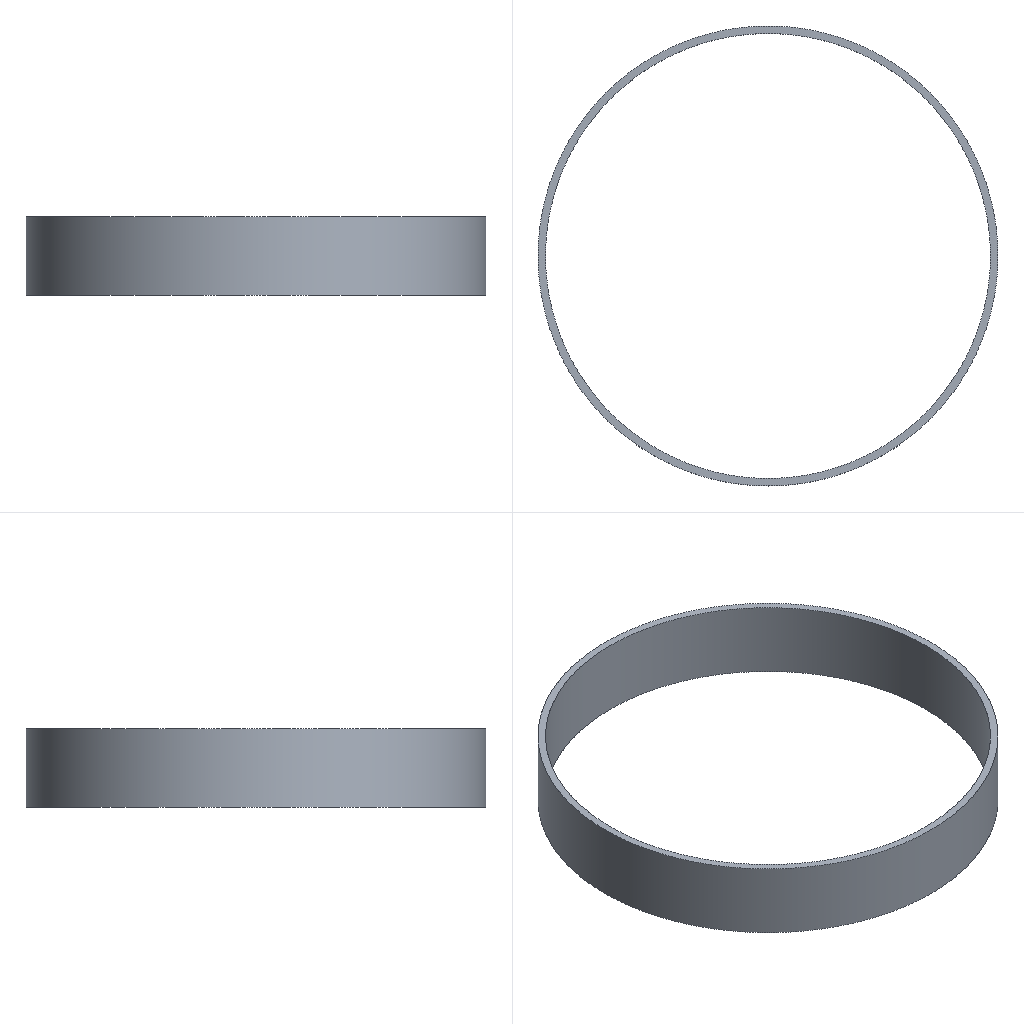Simulation study | abaqus
Set-up summary:
category,name,step,type,value,unit,region
solver,abaqus,,Abaqus/CAE 2024
units,SI m-kg-s (Pa),,inferred,E=8.17706e+09 density=500
analysis,Step-1,,frequency (modal),n_modes=10
mesh,nodes,,,220353
mesh,elements,,,176802
element_type,C3D8R,,,161472
element_type,B31,,,15038
element_type,CONN3D2,,,292
material,mucai,,E,8.17706e+09
material,mucai,,nu,0.3
material,mucai,,density,500
material,mucai,,yield,7.717e+07
material,mucai,,behaviors,plastic
material,tu,,E,1.3067e+08
material,tu,,nu,0.3
material,tu,,density,1624
material,tu,,behaviors,plastic; mohr coulomb; mohr coulomb hardening
section,tu,,solid section,,,Set-1
section,mucai,,beam section,,,_I1
section,mucai,,beam section,,,_I2
section,mucai,,beam section,,,_I3
bc,BC-1,initial,fixed,"[dofs=rx,ry,rz,x,y,z n=6]",,Set-1
constraint,connector section,,,1
Abaqus input file, long lists of numbers shortened:
*Heading
** Job name: deck Model name: motai
** Generated by: Abaqus/CAE 2024
*Preprint, echo=NO, model=NO, history=NO, contact=NO
**
** PARTS
**
*Part, name=Part-1
*Node
      1,           0.,   35.3,    3.1
      2,           0.,         36.5,    3.1
** (206043 more lines like these left out)
*Element, type=C3D8R
  1,    812,  16238, 104670,  15996,      1,    735,  15930,    762
  2,  16238,  16239, 104671, 104670,    735,    736,  15931,  15930
** (161470 more lines like these left out)
*Nset, nset=Set-1, generate
      1,  206045,       1
*Elset, elset=Set-1, generate
      1,  161472,       1
*Nset, nset=Set-100
      1,      4,      5,      8,      9,     11,     13,     15,     17,     19,     21,     23,     25,     27,     29,     31
     33,     35,     37,     39,     41,     43,     45,     47,     49,     51,     53,     55,     57,     59,     61,     63
** (2574 more lines like these left out)
** Section: tu
*Solid Section, elset=Set-1, material=tu
,
*End Part
**
*Part, name=Part-5
*Node
      1,  -3.908,  -30.097,    3.1
      2,  -3.908,  -30.097,           0.
** (14306 more lines like these left out)
*Element, type=B31
 1,   1, 958
 2, 958, 959
** (15036 more lines like these left out)
*Nset, nset=_PickedSet5, internal, generate
     1,  14308,      1
*Elset, elset=_PickedSet5, internal, generate
     1,  15038,      1
*Nset, nset=Set-4
     5,     6,     7,     8,     9,    10,    12,    13,    14,    15,    16,    18,    19,    22,    23,    24
    26,    27,    28,    29,    37,    38,    39,    40,    41,    42,    44,    45,    46,    49,    50,    51
** (259 more lines like these left out)
*Elset, elset=Set-4
    61,    62,    63,    64,    65,    66,    67,    68,    69,    70,    71,    72,    73,   118,   119,   120
   121,   122,   123,   124,   125,   126,   127,   128,   129,   130,   155,   156,   157,   158,   159,   160
** (241 more lines like these left out)
*Nset, nset=Set-3
     1,     2,     3,     4,     5,     6,     7,     8,    10,    11,    12,    13,    14,    16,    17,    20
    21,    22,    23,    25,    27,    28,    30,    31,    32,    33,    34,    35,    36,    37,    38,    39
** (322 more lines like these left out)
*Elset, elset=Set-3
     1,     2,     3,     4,     5,     6,     7,     8,     9,    10,    20,    21,    22,    23,    24,    25
    26,    27,    28,    29,    42,    43,    44,    45,    46,    47,    48,    49,    50,    51,    77,    78
** (313 more lines like these left out)
*Nset, nset=Set-100
     9,    15,    19,    24,    26,    29,    41,    42,    45,    46,    51,    52,    57,    58,    59,    71
    73,    76,    81,    82,    86,    89,    91,    92,    93,   105,   109,   114,   115,   118,   119,   120
** (73 more lines like these left out)
** Region: (Section-2:Picked), (Beam Orientation:Picked)
*Elset, elset=_I1, internal
     1,     2,     3,     4,     5,     6,     7,     8,     9,    10,    20,    21,    22,    23,    24,    25
    26,    27,    28,    29,    42,    43,    44,    45,    46,    47,    48,    49,    50,    51,    77,    78
** (318 more lines like these left out)
** Section: Section-2  Profile: Profile-1
*Beam Section, elset=_I1, material=mucai, temperature=GRADIENTS, section=CIRC
0.1
0.,1.,0.
** Region: (Section-2:Picked), (Beam Orientation:Picked)
*Elset, elset=_I2, internal
    11,    12,    13,    14,    15,    16,    17,    18,    19,    30,    31,    32,    33,    34,    35,    36
    37,    38,    39,    40,    41,    52,    53,    54,    55,    56,    57,    58,    59,    60,    74,    75
** (382 more lines like these left out)
** Section: Section-2  Profile: Profile-1
*Beam Section, elset=_I2, material=mucai, temperature=GRADIENTS, section=CIRC
0.1
0.,0.,-1.
** Region: (Section-2:Picked), (Beam Orientation:Set-4)
*Elset, elset=_I3, internal
    61,    62,    63,    64,    65,    66,    67,    68,    69,    70,    71,    72,    73,   118,   119,   120
   121,   122,   123,   124,   125,   126,   127,   128,   129,   130,   155,   156,   157,   158,   159,   160
** (236 more lines like these left out)
** Section: Section-2  Profile: Profile-1
*Beam Section, elset=_I3, material=mucai, temperature=GRADIENTS, section=CIRC
0.1
0.,0.,-1.
*End Part
**
**
** ASSEMBLY
**
*Assembly, name=Assembly
**
*Instance, name=Part-1-1, part=Part-1
*End Instance
**
*Instance, name=Part-5-1, part=Part-5
*End Instance
**
*Element, type=CONN3D2
1, Part-1-1.585, Part-5-1.29
2, Part-1-1.583, Part-5-1.58
** (290 more lines like these left out)
*Connector Section, elset=Wire-1-Set-2, behavior=ConnSect-1
Translator,
"Datum csys-2",
*Nset, nset=Set-1, instance=Part-1-1
    587,    588,    589,    590,    591,    592,    593,    594,    595,    596,    597,    598,    599,    600,    601,    602
    603,    604,    605,    606,    607,    608,    609,    610,    611,    612,    613,    614,    615,    616,    617,    618
** (261 more lines like these left out)
*Nset, nset=Set-1, instance=Part-5-1
  43,  72,  84, 106, 107, 133, 134, 136, 172, 173, 185, 211, 212, 239, 240, 242
 277, 278, 290, 316, 317, 344, 345, 346, 381, 382, 394, 420, 421, 448, 449, 450
** (3 more lines like these left out)
*Elset, elset=Set-1, instance=Part-1-1
 120529, 120530, 120531, 120532, 120533, 120534, 120535, 120536, 120537, 120538, 120539, 120540, 120541, 120542, 120543, 120544
 120545, 120546, 120547, 120548, 120549, 120550, 120551, 120552, 120553, 120554, 120555, 120556, 120557, 120558, 120559, 120560
** (209 more lines like these left out)
*Nset, nset=Wire-1-Set-2, instance=Part-1-1
   1,   4,   5,   8,   9,  11,  13,  15,  17,  19,  21,  23,  25,  27,  29,  31
  33,  35,  37,  39,  41,  43,  45,  47,  49,  51,  53,  55,  57,  59,  61,  63
** (17 more lines like these left out)
*Nset, nset=Wire-1-Set-2, instance=Part-5-1
   9,  15,  19,  24,  26,  29,  41,  42,  45,  46,  51,  52,  57,  58,  59,  71
  73,  76,  81,  82,  86,  89,  91,  92,  93, 105, 109, 114, 115, 118, 119, 120
** (17 more lines like these left out)
*Elset, elset=Wire-1-Set-2, generate
   1,  292,    1
*Orientation, name="Datum csys-2", system=CYLINDRICAL
5.77285490521717e-08,           0.,           0., 5.77285490521717e-08,           0.,           1.
1, 0.
*End Assembly
*Connector Behavior, name=ConnSect-1
*Connector Elasticity, component=1
 1e+08,
*Amplitude, name=Amp-1
             0.,              0.,            0.02,          0.0146,            0.04,          0.0118,            0.06,           0.009
           0.08,          0.0064,             0.1,          0.0048,            0.12,          0.0126,            0.14,          0.0205
           0.16,          0.0199,            0.18,          0.0132,             0.2,          0.0062,            0.22,         -0.0008
           0.24,          0.0134,            0.26,           0.028,            0.28,          0.0401,             0.3,          0.0311
           0.32,          0.0221,            0.34,          0.0129,            0.36,          0.0039,            0.38,          -0.005
            0.4,          -0.007,            0.42,          0.0126,            0.44,          0.0319,            0.46,          0.0485
           0.48,           0.012,             0.5,         -0.0247,            0.52,         -0.0611,            0.54,         -0.0291
           0.56,          0.0235,            0.58,           0.028,             0.6,          0.0339,            0.62,          0.0521
           0.64,          0.0701,            0.66,          0.0821,            0.68,          0.0403,             0.7,          0.0294
           0.72,          0.0286,            0.74,          0.0275,            0.76,          0.0095,            0.78,         -0.0221
            0.8,         -0.0541,            0.82,         -0.0902,            0.84,          -0.095,            0.86,         -0.1079
           0.88,         -0.1418,             0.9,         -0.1723,            0.92,         -0.1479,            0.94,         -0.1241
           0.96,            -0.1,            0.98,         -0.0757,              1.,         -0.1031,            1.02,         -0.1334
           1.04,         -0.1639,            1.06,         -0.1973,            1.08,         -0.2306,             1.1,         -0.2172
           1.12,         -0.1953,            1.14,         -0.1454,            1.16,         -0.1199,            1.18,         -0.0709
            1.2,          0.0874,            1.22,           0.246,            1.24,          0.1925,            1.26,          0.1281
           1.28,          0.0636,             1.3,          0.0017,            1.32,         -0.0496,            1.34,         -0.1012
           1.36,         -0.1527,            1.38,         -0.2113,             1.4,         -0.2858,            1.42,         -0.3629
           1.44,         -0.4371,            1.46,         -0.4629,            1.48,         -0.3743,             1.5,         -0.2886
           1.52,         -0.2578,            1.54,         -0.2768,            1.56,         -0.2687,            1.58,         -0.2603
            1.6,         -0.2973,            1.62,         -0.3402,            1.64,         -0.2256,            1.66,          0.2631
           1.68,          0.6714,             1.7,          0.6173,            1.72,          0.5657,            1.74,          0.5144
           1.76,          0.4629,            1.78,          0.4744,             1.8,          0.4859,            1.82,          0.4943
           1.84,          0.4716,            1.86,          0.3886,            1.88,          0.3029,             1.9,          0.2183
           1.92,           0.123,            1.94,          0.0076,            1.96,         -0.1079,            1.98,          -0.223
             2.,         -0.3371,            2.02,         -0.4542,            2.04,         -0.5685,            2.06,         -0.6828
           2.08,         -0.7972,             2.1,         -0.8714,            2.12,         -0.9345,            2.14,             -1.
           2.16,         -0.8972,            2.18,         -0.6971,             2.2,         -0.0154,            2.22,          0.7801
           2.24,          0.6344,            2.26,          0.4887,            2.28,           0.343,             2.3,          0.1989
           2.32,          0.0535,            2.34,          -0.049,            2.36,         -0.1519,            2.38,         -0.2541
            2.4,         -0.3573,            2.42,         -0.4601,            2.44,         -0.5629,            2.46,          0.6372
           2.48,          0.6686,             2.5,          0.4943,            2.52,            0.32,            2.54,          0.1451
           2.56,         -0.0291,            2.58,           0.021,             2.6,          0.4887,            2.62,          0.5542
           2.64,          0.4859,            2.66,          0.4172,            2.68,          0.3486,             2.7,          0.2796
           2.72,          0.2113,            2.74,          0.1429,            2.76,          0.0743,            2.78,          0.0059
            2.8,         -0.0625,            2.82,         -0.0286,            2.84,          0.0894,            2.86,          0.2071
           2.88,          0.2886,             2.9,          0.2247,            2.92,          0.1603,            2.94,          0.0961
           2.96,          0.0252,            2.98,          -0.051,              3.,         -0.1272,            3.02,         -0.2031
           3.04,         -0.0776,            3.06,          0.1323,            3.08,          0.0574,             3.1,         -0.0171
           3.12,         -0.0919,            3.14,         -0.1698,            3.16,         -0.2485,            3.18,         -0.3287
** (211 more lines like these left out)
**
** MATERIALS
**
*Material, name=mucai
*Density
500.,
*Elastic
 8.17706e+09, 0.3
*Plastic
 7.717e+07,0.
*Material, name=tu
*Density
1624.,
*Elastic
 1.3067e+08, 0.3
*Mohr Coulomb
39., 0.1
*Mohr Coulomb Hardening
140000.,0.
**
** BOUNDARY CONDITIONS
**
** Name: BC-1 Type: Displacement/Rotation
*Boundary
Set-1, 1, 1
Set-1, 2, 2
Set-1, 3, 3
Set-1, 4, 4
Set-1, 5, 5
Set-1, 6, 6
** ----------------------------------------------------------------
**
** STEP: Step-1
**
*Step, name=Step-1, nlgeom=NO, perturbation
*Frequency, eigensolver=Lanczos, sim, acoustic coupling=on, normalization=mass
10, , , , ,
**
** OUTPUT REQUESTS
**
*Restart, write, frequency=0
**
** FIELD OUTPUT: F-Output-1
**
*Output, field
*Node Output
U,
*End Step
Results summary:
result,odb.job_status,,,JOB_STATUS_COMPLETED_SUCCESSFULLY,"consistent, unstated (Abaqus has no unit system)"
result,steps[0].procedure,Step-1,,*FREQUENCY,"consistent, unstated (Abaqus has no unit system)"
result,steps[0].time_period,Step-1,,0,"consistent, unstated (Abaqus has no unit system)"
result,steps[0].n_frames,Step-1,,11,"consistent, unstated (Abaqus has no unit system)"
result,steps[0].last_frame.id,Step-1,,1,"consistent, unstated (Abaqus has no unit system)"
result,steps[0].last_frame.value,Step-1,,10,"consistent, unstated (Abaqus has no unit system)"
result,steps[0].last_frame.description,Step-1,,Mode        10: Value =   47.571     Freq =   1.098     (cycles/time),"consistent, unstated (Abaqus has no unit system)"
result,steps[0].max_U_magnitude,Step-1,,0.001138,"consistent, unstated (Abaqus has no unit system)"
result,steps[0].eigenfrequencies_hz[1],Step-1,,0.9142,"consistent, unstated (Abaqus has no unit system)"
result,steps[0].eigenfrequencies_hz[2],Step-1,,0.9142,"consistent, unstated (Abaqus has no unit system)"
result,steps[0].eigenfrequencies_hz[3],Step-1,,0.9197,"consistent, unstated (Abaqus has no unit system)"
result,steps[0].eigenfrequencies_hz[4],Step-1,,0.9197,"consistent, unstated (Abaqus has no unit system)"
result,steps[0].eigenfrequencies_hz[5],Step-1,,0.9744,"consistent, unstated (Abaqus has no unit system)"
result,steps[0].eigenfrequencies_hz[6],Step-1,,0.9745,"consistent, unstated (Abaqus has no unit system)"
result,steps[0].eigenfrequencies_hz[7],Step-1,,0.9844,"consistent, unstated (Abaqus has no unit system)"
result,steps[0].eigenfrequencies_hz[8],Step-1,,0.9844,"consistent, unstated (Abaqus has no unit system)"
result,steps[0].eigenfrequencies_hz[9],Step-1,,1.098,"consistent, unstated (Abaqus has no unit system)"
result,steps[0].eigenfrequencies_hz[10],Step-1,,1.098,"consistent, unstated (Abaqus has no unit system)"